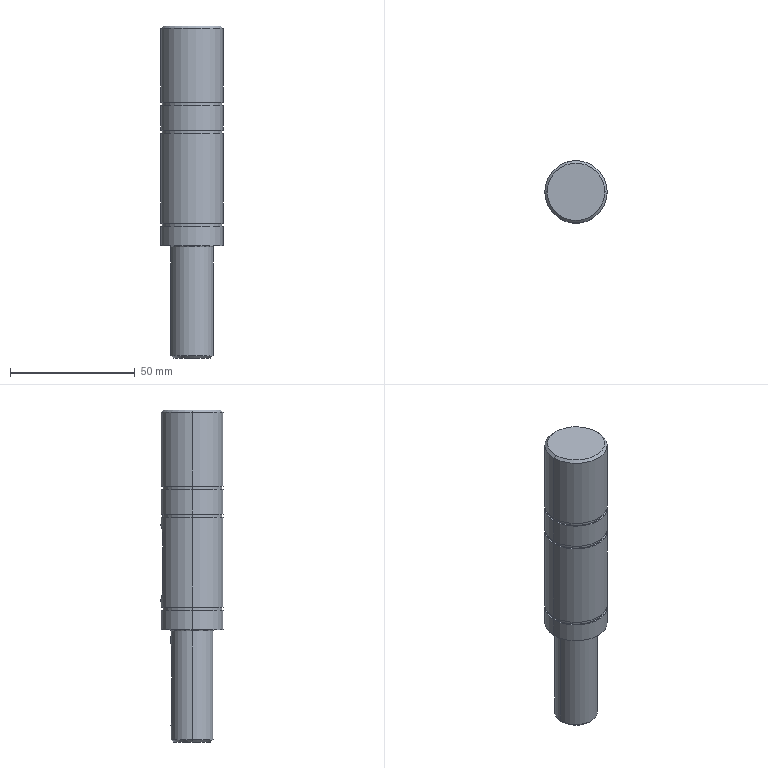Part | SolidWorks | features BaseBody 1 | 1 solid | 43 faces | box 25 x 25 x 133 mm | volume 51867 mm3 | cylinder 22 | plane 15 | cone 4 | spline 2 | commonest cylinder face diameters 25 x8 23.9 x6 5 x3 8 x3 17 x2
STEP:
#1=CARTESIAN_POINT('',(-8.5,0.,-0.5));
#2=VERTEX_POINT('',#1);
#3=CARTESIAN_POINT('',(8.5,0.,-0.5));
#4=VERTEX_POINT('',#3);
#5=CARTESIAN_POINT('',(0.,0.,-0.5));
#6=DIRECTION('',(0.,0.,-1.));
#7=DIRECTION('',(1.,0.,0.));
#8=AXIS2_PLACEMENT_3D('',#5,#6,#7);
#9=CIRCLE('',#8,8.5);
#10=EDGE_CURVE('',#2,#4,#9,.T.);
#11=ORIENTED_EDGE('',*,*,#10,.F.);
#12=CARTESIAN_POINT('',(-9.,0.,0.));
#13=VERTEX_POINT('',#12);
#14=CARTESIAN_POINT('',(-9.,0.,-0.5));
#15=DIRECTION('',(0.,-1.,0.));
#16=DIRECTION('',(-1.,0.,0.));
#17=AXIS2_PLACEMENT_3D('',#14,#15,#16);
#18=CIRCLE('',#17,0.5);
#19=EDGE_CURVE('',#2,#13,#18,.T.);
#20=ORIENTED_EDGE('',*,*,#19,.T.);
#21=CARTESIAN_POINT('',(9.,0.,0.));
#22=VERTEX_POINT('',#21);
#23=CARTESIAN_POINT('',(-9.,0.,0.));
#24=CARTESIAN_POINT('',(-9.,18.,0.));
#25=CARTESIAN_POINT('',(9.,18.,0.));
#26=CARTESIAN_POINT('',(9.,0.,0.));
#27=(BOUNDED_CURVE()B_SPLINE_CURVE(3,(#23,#24,#25,#26),.UNSPECIFIED.,.F.,.F.)B_SPLINE_CURVE_WITH_KNOTS((4,4),(0.,1.),.UNSPECIFIED.)CURVE()GEOMETRIC_REPRESENTATION_ITEM()RATIONAL_B_SPLINE_CURVE((1.,0.3333,0.3333,1.))REPRESENTATION_ITEM(''));
#28=EDGE_CURVE('',#13,#22,#27,.T.);
#29=ORIENTED_EDGE('',*,*,#28,.T.);
#30=CARTESIAN_POINT('',(9.,0.,-0.5));
#31=DIRECTION('',(0.,1.,0.));
#32=DIRECTION('',(1.,0.,0.));
#33=AXIS2_PLACEMENT_3D('',#30,#31,#32);
#34=CIRCLE('',#33,0.5);
#35=EDGE_CURVE('',#4,#22,#34,.T.);
#36=ORIENTED_EDGE('',*,*,#35,.F.);
#37=EDGE_LOOP('',(#11,#20,#29,#36));
#38=FACE_OUTER_BOUND('',#37,.T.);
#39=CARTESIAN_POINT('',(8.5,0.,-0.5));
#40=CARTESIAN_POINT('',(8.5,17.,-0.5));
#41=CARTESIAN_POINT('',(-8.5,17.,-0.5));
#42=CARTESIAN_POINT('',(-8.5,0.,-0.5));
#43=CARTESIAN_POINT('',(8.5,0.,-0.2071));
#44=CARTESIAN_POINT('',(8.5,17.,-0.2071));
#45=CARTESIAN_POINT('',(-8.5,17.,-0.2071));
#46=CARTESIAN_POINT('',(-8.5,0.,-0.2071));
#47=CARTESIAN_POINT('',(8.707,0.,0.));
#48=CARTESIAN_POINT('',(8.707,17.414,0.));
#49=CARTESIAN_POINT('',(-8.707,17.414,0.));
#50=CARTESIAN_POINT('',(-8.707,0.,0.));
#51=CARTESIAN_POINT('',(9.,0.,0.));
#52=CARTESIAN_POINT('',(9.,18.,0.));
#53=CARTESIAN_POINT('',(-9.,18.,0.));
#54=CARTESIAN_POINT('',(-9.,0.,0.));
#55=(BOUNDED_SURFACE()B_SPLINE_SURFACE(3,3,((#39,#40,#41,#42),(#43,#44,#45,#46),(#47,#48,#49,#50),(#51,#52,#53,#54)),.UNSPECIFIED.,.F.,.F.,.T.)B_SPLINE_SURFACE_WITH_KNOTS((4,4),(4,4),(0.,1.),(0.,1.),.UNSPECIFIED.)GEOMETRIC_REPRESENTATION_ITEM()RATIONAL_B_SPLINE_SURFACE(((1.,0.3333,0.3333,1.),(0.8047,0.2682,0.2682,0.8047),(0.8047,0.2682,0.2682,0.8047),(1.,0.3333,0.3333,1.)))REPRESENTATION_ITEM('')SURFACE());
#56=ADVANCED_FACE('',(#38),#55,.F.);
#57=CARTESIAN_POINT('',(-4.,11.843,16.));
#58=VERTEX_POINT('',#57);
#59=CARTESIAN_POINT('',(0.,12.5,12.));
#60=VERTEX_POINT('',#59);
#61=CARTESIAN_POINT('',(-4.,11.843,16.));
#62=CARTESIAN_POINT('',(-4.,11.843,15.734));
#63=CARTESIAN_POINT('',(-3.974,11.852,15.473));
#64=CARTESIAN_POINT('',(-3.871,11.886,14.96));
#65=CARTESIAN_POINT('',(-3.794,11.911,14.705));
#66=CARTESIAN_POINT('',(-3.592,11.973,14.221));
#67=CARTESIAN_POINT('',(-3.47,12.01,13.993));
#68=CARTESIAN_POINT('',(-3.18,12.09,13.559));
#69=CARTESIAN_POINT('',(-3.012,12.133,13.356));
#70=CARTESIAN_POINT('',(-2.646,12.218,12.989));
#71=CARTESIAN_POINT('',(-2.446,12.26,12.824));
#72=CARTESIAN_POINT('',(-2.01,12.339,12.532));
#73=CARTESIAN_POINT('',(-1.78,12.375,12.409));
#74=CARTESIAN_POINT('',(-1.3,12.435,12.208));
#75=CARTESIAN_POINT('',(-1.047,12.459,12.13));
#76=CARTESIAN_POINT('',(-0.5285,12.492,12.026));
#77=CARTESIAN_POINT('',(-0.266,12.5,12.));
#78=CARTESIAN_POINT('',(0.,12.5,12.));
#79=B_SPLINE_CURVE_WITH_KNOTS('',3,(#61,#62,#63,#64,#65,#66,#67,#68,#69,#70,#71,#72,#73,#74,#75,#76,#77,#78),.UNSPECIFIED.,.F.,.F.,(4,2,2,2,2,2,2,2,4),(-0.00629,-0.005504,-0.004718,-0.003932,-0.003145,-0.002359,-0.001573,-0.0007863,0.),.UNSPECIFIED.);
#80=EDGE_CURVE('',#58,#60,#79,.T.);
#81=ORIENTED_EDGE('',*,*,#80,.T.);
#82=CARTESIAN_POINT('',(4.,11.843,16.));
#83=VERTEX_POINT('',#82);
#84=CARTESIAN_POINT('',(0.,12.5,12.));
#85=CARTESIAN_POINT('',(0.266,12.5,12.));
#86=CARTESIAN_POINT('',(0.5272,12.492,12.026));
#87=CARTESIAN_POINT('',(1.041,12.459,12.129));
#88=CARTESIAN_POINT('',(1.296,12.435,12.207));
#89=CARTESIAN_POINT('',(1.779,12.375,12.408));
#90=CARTESIAN_POINT('',(2.008,12.34,12.531));
#91=CARTESIAN_POINT('',(2.441,12.261,12.821));
#92=CARTESIAN_POINT('',(2.645,12.218,12.988));
#93=CARTESIAN_POINT('',(3.011,12.133,13.354));
#94=CARTESIAN_POINT('',(3.176,12.091,13.554));
#95=CARTESIAN_POINT('',(3.469,12.01,13.991));
#96=CARTESIAN_POINT('',(3.592,11.973,14.22));
#97=CARTESIAN_POINT('',(3.792,11.911,14.7));
#98=CARTESIAN_POINT('',(3.87,11.886,14.954));
#99=CARTESIAN_POINT('',(3.974,11.852,15.472));
#100=CARTESIAN_POINT('',(4.,11.843,15.734));
#101=CARTESIAN_POINT('',(4.,11.843,16.));
#102=B_SPLINE_CURVE_WITH_KNOTS('',3,(#84,#85,#86,#87,#88,#89,#90,#91,#92,#93,#94,#95,#96,#97,#98,#99,#100,#101),.UNSPECIFIED.,.F.,.F.,(4,2,2,2,2,2,2,2,4),(0.,0.0007863,0.001573,0.002359,0.003145,0.003932,0.004718,0.005504,0.00629),.UNSPECIFIED.);
#103=EDGE_CURVE('',#60,#83,#102,.T.);
#104=ORIENTED_EDGE('',*,*,#103,.T.);
#105=CARTESIAN_POINT('',(4.,11.843,38.));
#106=VERTEX_POINT('',#105);
#107=CARTESIAN_POINT('',(4.,11.843,88.));
#108=DIRECTION('',(0.,0.,1.));
#109=VECTOR('',#108,1000.);
#110=LINE('',#107,#109);
#111=EDGE_CURVE('',#83,#106,#110,.T.);
#112=ORIENTED_EDGE('',*,*,#111,.T.);
#113=CARTESIAN_POINT('',(-4.,11.843,38.));
#114=VERTEX_POINT('',#113);
#115=CARTESIAN_POINT('',(4.,11.843,38.));
#116=CARTESIAN_POINT('',(4.,11.843,38.266));
#117=CARTESIAN_POINT('',(3.974,11.852,38.527));
#118=CARTESIAN_POINT('',(3.871,11.886,39.041));
#119=CARTESIAN_POINT('',(3.793,11.911,39.296));
#120=CARTESIAN_POINT('',(3.592,11.973,39.779));
#121=CARTESIAN_POINT('',(3.469,12.01,40.008));
#122=CARTESIAN_POINT('',(3.179,12.09,40.441));
#123=CARTESIAN_POINT('',(3.012,12.133,40.645));
#124=CARTESIAN_POINT('',(2.646,12.218,41.011));
#125=CARTESIAN_POINT('',(2.445,12.26,41.176));
#126=CARTESIAN_POINT('',(2.009,12.34,41.469));
#127=CARTESIAN_POINT('',(1.779,12.375,41.592));
#128=CARTESIAN_POINT('',(1.299,12.435,41.792));
#129=CARTESIAN_POINT('',(1.045,12.459,41.87));
#130=CARTESIAN_POINT('',(0.5276,12.492,41.974));
#131=CARTESIAN_POINT('',(0.2669,12.5,42.));
#132=CARTESIAN_POINT('',(-0.2587,12.5,42.));
#133=CARTESIAN_POINT('',(-0.5256,12.492,41.974));
#134=CARTESIAN_POINT('',(-1.04,12.459,41.871));
#135=CARTESIAN_POINT('',(-1.29,12.436,41.795));
#136=CARTESIAN_POINT('',(-1.777,12.375,41.593));
#137=CARTESIAN_POINT('',(-2.008,12.34,41.469));
#138=CARTESIAN_POINT('',(-2.44,12.262,41.18));
#139=CARTESIAN_POINT('',(-2.643,12.219,41.013));
#140=CARTESIAN_POINT('',(-3.012,12.133,40.645));
#141=CARTESIAN_POINT('',(-3.176,12.091,40.445));
#142=CARTESIAN_POINT('',(-3.466,12.011,40.013));
#143=CARTESIAN_POINT('',(-3.592,11.973,39.78));
#144=CARTESIAN_POINT('',(-3.792,11.911,39.298));
#145=CARTESIAN_POINT('',(-3.869,11.886,39.049));
#146=CARTESIAN_POINT('',(-3.973,11.852,38.532));
#147=CARTESIAN_POINT('',(-4.,11.843,38.266));
#148=CARTESIAN_POINT('',(-4.,11.843,38.));
#149=B_SPLINE_CURVE_WITH_KNOTS('',3,(#115,#116,#117,#118,#119,#120,#121,#122,#123,#124,#125,#126,#127,#128,#129,#130,#131,#132,#133,#134,#135,#136,#137,#138,#139,#140,#141,#142,#143,#144,#145,#146,#147,#148),.UNSPECIFIED.,.F.,.F.,(4,2,2,2,2,2,2,2,2,2,2,2,2,2,2,2,4),(0.,0.0007865,0.001573,0.00236,0.003146,0.003933,0.004719,0.005506,0.006292,0.007079,0.007865,0.008652,0.009438,0.01022,0.01101,0.0118,0.01258),.UNSPECIFIED.);
#150=EDGE_CURVE('',#106,#114,#149,.T.);
#151=ORIENTED_EDGE('',*,*,#150,.T.);
#152=CARTESIAN_POINT('',(-4.,11.843,88.));
#153=DIRECTION('',(0.,0.,-1.));
#154=VECTOR('',#153,1000.);
#155=LINE('',#152,#154);
#156=EDGE_CURVE('',#114,#58,#155,.T.);
#157=ORIENTED_EDGE('',*,*,#156,.T.);
#158=EDGE_LOOP('',(#81,#104,#112,#151,#157));
#159=FACE_BOUND('',#158,.T.);
#160=CARTESIAN_POINT('',(-12.5,0.,45.));
#161=VERTEX_POINT('',#160);
#162=CARTESIAN_POINT('',(12.5,0.,45.));
#163=VERTEX_POINT('',#162);
#164=CARTESIAN_POINT('',(0.,0.,45.));
#165=DIRECTION('',(0.,0.,-1.));
#166=DIRECTION('',(-1.,0.,0.));
#167=AXIS2_PLACEMENT_3D('',#164,#165,#166);
#168=CIRCLE('',#167,12.5);
#169=EDGE_CURVE('',#161,#163,#168,.T.);
#170=ORIENTED_EDGE('',*,*,#169,.T.);
#171=CARTESIAN_POINT('',(12.5,0.,9.));
#172=VERTEX_POINT('',#171);
#173=CARTESIAN_POINT('',(12.5,0.,88.));
#174=DIRECTION('',(0.,0.,-1.));
#175=VECTOR('',#174,1000.);
#176=LINE('',#173,#175);
#177=EDGE_CURVE('',#163,#172,#176,.T.);
#178=ORIENTED_EDGE('',*,*,#177,.T.);
#179=CARTESIAN_POINT('',(-12.5,0.,9.));
#180=VERTEX_POINT('',#179);
#181=CARTESIAN_POINT('',(0.,0.,9.));
#182=DIRECTION('',(0.,0.,1.));
#183=DIRECTION('',(-1.,0.,0.));
#184=AXIS2_PLACEMENT_3D('',#181,#182,#183);
#185=CIRCLE('',#184,12.5);
#186=EDGE_CURVE('',#172,#180,#185,.T.);
#187=ORIENTED_EDGE('',*,*,#186,.T.);
#188=CARTESIAN_POINT('',(-12.5,0.,88.));
#189=DIRECTION('',(0.,0.,-1.));
#190=VECTOR('',#189,1000.);
#191=LINE('',#188,#190);
#192=EDGE_CURVE('',#161,#180,#191,.T.);
#193=ORIENTED_EDGE('',*,*,#192,.F.);
#194=EDGE_LOOP('',(#170,#178,#187,#193));
#195=FACE_OUTER_BOUND('',#194,.T.);
#196=CARTESIAN_POINT('',(0.,0.,88.));
#197=DIRECTION('',(0.,0.,-1.));
#198=DIRECTION('',(-1.,0.,0.));
#199=AXIS2_PLACEMENT_3D('',#196,#197,#198);
#200=CYLINDRICAL_SURFACE('',#199,12.5);
#201=ADVANCED_FACE('',(#159,#195),#200,.T.);
#202=CARTESIAN_POINT('',(-11.95,0.,9.));
#203=VERTEX_POINT('',#202);
#204=CARTESIAN_POINT('',(11.95,0.,9.));
#205=VERTEX_POINT('',#204);
#206=CARTESIAN_POINT('',(0.,0.,9.));
#207=DIRECTION('',(0.,0.,-1.));
#208=DIRECTION('',(-1.,0.,0.));
#209=AXIS2_PLACEMENT_3D('',#206,#207,#208);
#210=CIRCLE('',#209,11.95);
#211=EDGE_CURVE('',#203,#205,#210,.T.);
#212=ORIENTED_EDGE('',*,*,#211,.T.);
#213=CARTESIAN_POINT('',(11.95,0.,7.7));
#214=VERTEX_POINT('',#213);
#215=CARTESIAN_POINT('',(11.95,0.,0.));
#216=DIRECTION('',(0.,0.,-1.));
#217=VECTOR('',#216,1000.);
#218=LINE('',#215,#217);
#219=EDGE_CURVE('',#205,#214,#218,.T.);
#220=ORIENTED_EDGE('',*,*,#219,.T.);
#221=CARTESIAN_POINT('',(-11.95,0.,7.7));
#222=VERTEX_POINT('',#221);
#223=CARTESIAN_POINT('',(0.,0.,7.7));
#224=DIRECTION('',(0.,0.,1.));
#225=DIRECTION('',(-1.,0.,0.));
#226=AXIS2_PLACEMENT_3D('',#223,#224,#225);
#227=CIRCLE('',#226,11.95);
#228=EDGE_CURVE('',#214,#222,#227,.T.);
#229=ORIENTED_EDGE('',*,*,#228,.T.);
#230=CARTESIAN_POINT('',(-11.95,0.,0.));
#231=DIRECTION('',(0.,0.,-1.));
#232=VECTOR('',#231,1000.);
#233=LINE('',#230,#232);
#234=EDGE_CURVE('',#203,#222,#233,.T.);
#235=ORIENTED_EDGE('',*,*,#234,.F.);
#236=EDGE_LOOP('',(#212,#220,#229,#235));
#237=FACE_OUTER_BOUND('',#236,.T.);
#238=CARTESIAN_POINT('',(0.,0.,0.));
#239=DIRECTION('',(0.,0.,-1.));
#240=DIRECTION('',(-1.,0.,0.));
#241=AXIS2_PLACEMENT_3D('',#238,#239,#240);
#242=CYLINDRICAL_SURFACE('',#241,11.95);
#243=ADVANCED_FACE('',(#237),#242,.T.);
#244=ORIENTED_EDGE('',*,*,#103,.F.);
#245=CARTESIAN_POINT('',(0.,8.5,12.));
#246=VERTEX_POINT('',#245);
#247=CARTESIAN_POINT('',(0.,12.5,12.));
#248=DIRECTION('',(0.,-1.,0.));
#249=VECTOR('',#248,1000.);
#250=LINE('',#247,#249);
#251=EDGE_CURVE('',#60,#246,#250,.T.);
#252=ORIENTED_EDGE('',*,*,#251,.T.);
#253=CARTESIAN_POINT('',(4.,8.5,16.));
#254=VERTEX_POINT('',#253);
#255=CARTESIAN_POINT('',(0.,8.5,16.));
#256=DIRECTION('',(0.,1.,0.));
#257=DIRECTION('',(0.,0.,-1.));
#258=AXIS2_PLACEMENT_3D('',#255,#256,#257);
#259=CIRCLE('',#258,4.);
#260=EDGE_CURVE('',#254,#246,#259,.T.);
#261=ORIENTED_EDGE('',*,*,#260,.F.);
#262=CARTESIAN_POINT('',(4.,12.5,16.));
#263=DIRECTION('',(0.,-1.,0.));
#264=VECTOR('',#263,1000.);
#265=LINE('',#262,#264);
#266=EDGE_CURVE('',#83,#254,#265,.T.);
#267=ORIENTED_EDGE('',*,*,#266,.F.);
#268=EDGE_LOOP('',(#244,#252,#261,#267));
#269=FACE_OUTER_BOUND('',#268,.T.);
#270=CARTESIAN_POINT('',(0.,12.5,16.));
#271=DIRECTION('',(0.,-1.,0.));
#272=DIRECTION('',(0.,0.,-1.));
#273=AXIS2_PLACEMENT_3D('',#270,#271,#272);
#274=CYLINDRICAL_SURFACE('',#273,4.);
#275=ADVANCED_FACE('',(#269),#274,.F.);
#276=CARTESIAN_POINT('',(-11.95,0.,46.3));
#277=VERTEX_POINT('',#276);
#278=CARTESIAN_POINT('',(11.95,0.,46.3));
#279=VERTEX_POINT('',#278);
#280=CARTESIAN_POINT('',(0.,0.,46.3));
#281=DIRECTION('',(0.,0.,-1.));
#282=DIRECTION('',(-1.,0.,0.));
#283=AXIS2_PLACEMENT_3D('',#280,#281,#282);
#284=CIRCLE('',#283,11.95);
#285=EDGE_CURVE('',#277,#279,#284,.T.);
#286=ORIENTED_EDGE('',*,*,#285,.T.);
#287=CARTESIAN_POINT('',(11.95,0.,45.));
#288=VERTEX_POINT('',#287);
#289=CARTESIAN_POINT('',(11.95,0.,0.));
#290=DIRECTION('',(0.,0.,-1.));
#291=VECTOR('',#290,1000.);
#292=LINE('',#289,#291);
#293=EDGE_CURVE('',#279,#288,#292,.T.);
#294=ORIENTED_EDGE('',*,*,#293,.T.);
#295=CARTESIAN_POINT('',(-11.95,0.,45.));
#296=VERTEX_POINT('',#295);
#297=CARTESIAN_POINT('',(0.,0.,45.));
#298=DIRECTION('',(0.,0.,1.));
#299=DIRECTION('',(-1.,0.,0.));
#300=AXIS2_PLACEMENT_3D('',#297,#298,#299);
#301=CIRCLE('',#300,11.95);
#302=EDGE_CURVE('',#288,#296,#301,.T.);
#303=ORIENTED_EDGE('',*,*,#302,.T.);
#304=CARTESIAN_POINT('',(-11.95,0.,0.));
#305=DIRECTION('',(0.,0.,-1.));
#306=VECTOR('',#305,1000.);
#307=LINE('',#304,#306);
#308=EDGE_CURVE('',#277,#296,#307,.T.);
#309=ORIENTED_EDGE('',*,*,#308,.F.);
#310=EDGE_LOOP('',(#286,#294,#303,#309));
#311=FACE_OUTER_BOUND('',#310,.T.);
#312=CARTESIAN_POINT('',(0.,0.,0.));
#313=DIRECTION('',(0.,0.,-1.));
#314=DIRECTION('',(-1.,0.,0.));
#315=AXIS2_PLACEMENT_3D('',#312,#313,#314);
#316=CYLINDRICAL_SURFACE('',#315,11.95);
#317=ADVANCED_FACE('',(#311),#316,.T.);
#318=CARTESIAN_POINT('',(-12.5,0.,7.7));
#319=VERTEX_POINT('',#318);
#320=CARTESIAN_POINT('',(12.5,0.,7.7));
#321=VERTEX_POINT('',#320);
#322=CARTESIAN_POINT('',(0.,0.,7.7));
#323=DIRECTION('',(0.,0.,-1.));
#324=DIRECTION('',(-1.,0.,0.));
#325=AXIS2_PLACEMENT_3D('',#322,#323,#324);
#326=CIRCLE('',#325,12.5);
#327=EDGE_CURVE('',#319,#321,#326,.T.);
#328=ORIENTED_EDGE('',*,*,#327,.T.);
#329=CARTESIAN_POINT('',(12.5,0.,0.));
#330=VERTEX_POINT('',#329);
#331=CARTESIAN_POINT('',(12.5,0.,88.));
#332=DIRECTION('',(0.,0.,-1.));
#333=VECTOR('',#332,1000.);
#334=LINE('',#331,#333);
#335=EDGE_CURVE('',#321,#330,#334,.T.);
#336=ORIENTED_EDGE('',*,*,#335,.T.);
#337=CARTESIAN_POINT('',(-12.5,0.,0.));
#338=VERTEX_POINT('',#337);
#339=CARTESIAN_POINT('',(0.,0.,0.));
#340=DIRECTION('',(0.,0.,1.));
#341=DIRECTION('',(-1.,0.,0.));
#342=AXIS2_PLACEMENT_3D('',#339,#340,#341);
#343=CIRCLE('',#342,12.5);
#344=EDGE_CURVE('',#330,#338,#343,.T.);
#345=ORIENTED_EDGE('',*,*,#344,.T.);
#346=CARTESIAN_POINT('',(-12.5,0.,88.));
#347=DIRECTION('',(0.,0.,-1.));
#348=VECTOR('',#347,1000.);
#349=LINE('',#346,#348);
#350=EDGE_CURVE('',#319,#338,#349,.T.);
#351=ORIENTED_EDGE('',*,*,#350,.F.);
#352=EDGE_LOOP('',(#328,#336,#345,#351));
#353=FACE_OUTER_BOUND('',#352,.T.);
#354=CARTESIAN_POINT('',(0.,0.,88.));
#355=DIRECTION('',(0.,0.,-1.));
#356=DIRECTION('',(-1.,0.,0.));
#357=AXIS2_PLACEMENT_3D('',#354,#355,#356);
#358=CYLINDRICAL_SURFACE('',#357,12.5);
#359=ADVANCED_FACE('',(#353),#358,.T.);
#360=CARTESIAN_POINT('',(-12.5,0.,56.2));
#361=VERTEX_POINT('',#360);
#362=CARTESIAN_POINT('',(12.5,0.,56.2));
#363=VERTEX_POINT('',#362);
#364=CARTESIAN_POINT('',(0.,0.,56.2));
#365=DIRECTION('',(0.,0.,-1.));
#366=DIRECTION('',(-1.,0.,0.));
#367=AXIS2_PLACEMENT_3D('',#364,#365,#366);
#368=CIRCLE('',#367,12.5);
#369=EDGE_CURVE('',#361,#363,#368,.T.);
#370=ORIENTED_EDGE('',*,*,#369,.T.);
#371=CARTESIAN_POINT('',(12.5,0.,46.3));
#372=VERTEX_POINT('',#371);
#373=CARTESIAN_POINT('',(12.5,0.,88.));
#374=DIRECTION('',(0.,0.,-1.));
#375=VECTOR('',#374,1000.);
#376=LINE('',#373,#375);
#377=EDGE_CURVE('',#363,#372,#376,.T.);
#378=ORIENTED_EDGE('',*,*,#377,.T.);
#379=CARTESIAN_POINT('',(-12.5,0.,46.3));
#380=VERTEX_POINT('',#379);
#381=CARTESIAN_POINT('',(0.,0.,46.3));
#382=DIRECTION('',(0.,0.,1.));
#383=DIRECTION('',(-1.,0.,0.));
#384=AXIS2_PLACEMENT_3D('',#381,#382,#383);
#385=CIRCLE('',#384,12.5);
#386=EDGE_CURVE('',#372,#380,#385,.T.);
#387=ORIENTED_EDGE('',*,*,#386,.T.);
#388=CARTESIAN_POINT('',(-12.5,0.,88.));
#389=DIRECTION('',(0.,0.,-1.));
#390=VECTOR('',#389,1000.);
#391=LINE('',#388,#390);
#392=EDGE_CURVE('',#361,#380,#391,.T.);
#393=ORIENTED_EDGE('',*,*,#392,.F.);
#394=EDGE_LOOP('',(#370,#378,#387,#393));
#395=FACE_OUTER_BOUND('',#394,.T.);
#396=CARTESIAN_POINT('',(0.,0.,88.));
#397=DIRECTION('',(0.,0.,-1.));
#398=DIRECTION('',(-1.,0.,0.));
#399=AXIS2_PLACEMENT_3D('',#396,#397,#398);
#400=CYLINDRICAL_SURFACE('',#399,12.5);
#401=ADVANCED_FACE('',(#395),#400,.T.);
#402=CARTESIAN_POINT('',(-11.95,0.,57.5));
#403=VERTEX_POINT('',#402);
#404=CARTESIAN_POINT('',(11.95,0.,57.5));
#405=VERTEX_POINT('',#404);
#406=CARTESIAN_POINT('',(0.,0.,57.5));
#407=DIRECTION('',(0.,0.,-1.));
#408=DIRECTION('',(-1.,0.,0.));
#409=AXIS2_PLACEMENT_3D('',#406,#407,#408);
#410=CIRCLE('',#409,11.95);
#411=EDGE_CURVE('',#403,#405,#410,.T.);
#412=ORIENTED_EDGE('',*,*,#411,.T.);
#413=CARTESIAN_POINT('',(11.95,0.,56.2));
#414=VERTEX_POINT('',#413);
#415=CARTESIAN_POINT('',(11.95,0.,0.));
#416=DIRECTION('',(0.,0.,-1.));
#417=VECTOR('',#416,1000.);
#418=LINE('',#415,#417);
#419=EDGE_CURVE('',#405,#414,#418,.T.);
#420=ORIENTED_EDGE('',*,*,#419,.T.);
#421=CARTESIAN_POINT('',(-11.95,0.,56.2));
#422=VERTEX_POINT('',#421);
#423=CARTESIAN_POINT('',(0.,0.,56.2));
#424=DIRECTION('',(0.,0.,1.));
#425=DIRECTION('',(-1.,0.,0.));
#426=AXIS2_PLACEMENT_3D('',#423,#424,#425);
#427=CIRCLE('',#426,11.95);
#428=EDGE_CURVE('',#414,#422,#427,.T.);
#429=ORIENTED_EDGE('',*,*,#428,.T.);
#430=CARTESIAN_POINT('',(-11.95,0.,0.));
#431=DIRECTION('',(0.,0.,-1.));
#432=VECTOR('',#431,1000.);
#433=LINE('',#430,#432);
#434=EDGE_CURVE('',#403,#422,#433,.T.);
#435=ORIENTED_EDGE('',*,*,#434,.F.);
#436=EDGE_LOOP('',(#412,#420,#429,#435));
#437=FACE_OUTER_BOUND('',#436,.T.);
#438=CARTESIAN_POINT('',(0.,0.,0.));
#439=DIRECTION('',(0.,0.,-1.));
#440=DIRECTION('',(-1.,0.,0.));
#441=AXIS2_PLACEMENT_3D('',#438,#439,#440);
#442=CYLINDRICAL_SURFACE('',#441,11.95);
#443=ADVANCED_FACE('',(#437),#442,.T.);
#444=CARTESIAN_POINT('',(-2.5,8.124,-8.));
#445=VERTEX_POINT('',#444);
#446=CARTESIAN_POINT('',(-2.5,8.124,-36.));
#447=VERTEX_POINT('',#446);
#448=CARTESIAN_POINT('',(-2.5,8.124,-45.));
#449=DIRECTION('',(0.,0.,-1.));
#450=VECTOR('',#449,1000.);
#451=LINE('',#448,#450);
#452=EDGE_CURVE('',#445,#447,#451,.T.);
#453=ORIENTED_EDGE('',*,*,#452,.T.);
#454=CARTESIAN_POINT('',(0.,8.5,-38.5));
#455=VERTEX_POINT('',#454);
#456=CARTESIAN_POINT('',(-2.5,8.124,-36.));
#457=CARTESIAN_POINT('',(-2.5,8.124,-36.166));
#458=CARTESIAN_POINT('',(-2.484,8.129,-36.329));
#459=CARTESIAN_POINT('',(-2.42,8.148,-36.65));
#460=CARTESIAN_POINT('',(-2.371,8.163,-36.809));
#461=CARTESIAN_POINT('',(-2.246,8.198,-37.111));
#462=CARTESIAN_POINT('',(-2.169,8.219,-37.254));
#463=CARTESIAN_POINT('',(-1.988,8.265,-37.525));
#464=CARTESIAN_POINT('',(-1.883,8.29,-37.653));
#465=CARTESIAN_POINT('',(-1.539,8.363,-37.996));
#466=CARTESIAN_POINT('',(-1.262,8.411,-38.182));
#467=CARTESIAN_POINT('',(-0.8118,8.462,-38.37));
#468=CARTESIAN_POINT('',(-0.6536,8.476,-38.419));
#469=CARTESIAN_POINT('',(-0.33,8.495,-38.484));
#470=CARTESIAN_POINT('',(-0.1661,8.5,-38.5));
#471=CARTESIAN_POINT('',(0.,8.5,-38.5));
#472=B_SPLINE_CURVE_WITH_KNOTS('',3,(#456,#457,#458,#459,#460,#461,#462,#463,#464,#465,#466,#467,#468,#469,#470,#471),.UNSPECIFIED.,.F.,.F.,(4,2,2,2,2,2,2,4),(0.,0.0004909,0.0009818,0.001473,0.001964,0.002945,0.003436,0.003927),.UNSPECIFIED.);
#473=EDGE_CURVE('',#447,#455,#472,.T.);
#474=ORIENTED_EDGE('',*,*,#473,.T.);
#475=CARTESIAN_POINT('',(2.5,8.124,-36.));
#476=VERTEX_POINT('',#475);
#477=CARTESIAN_POINT('',(0.,8.5,-38.5));
#478=CARTESIAN_POINT('',(0.1661,8.5,-38.5));
#479=CARTESIAN_POINT('',(0.3292,8.495,-38.484));
#480=CARTESIAN_POINT('',(0.6498,8.477,-38.42));
#481=CARTESIAN_POINT('',(0.809,8.463,-38.371));
#482=CARTESIAN_POINT('',(1.111,8.428,-38.245));
#483=CARTESIAN_POINT('',(1.254,8.408,-38.169));
#484=CARTESIAN_POINT('',(1.525,8.363,-37.987));
#485=CARTESIAN_POINT('',(1.653,8.339,-37.883));
#486=CARTESIAN_POINT('',(1.997,8.265,-37.539));
#487=CARTESIAN_POINT('',(2.183,8.216,-37.262));
#488=CARTESIAN_POINT('',(2.37,8.163,-36.812));
#489=CARTESIAN_POINT('',(2.419,8.149,-36.654));
#490=CARTESIAN_POINT('',(2.484,8.129,-36.33));
#491=CARTESIAN_POINT('',(2.5,8.124,-36.166));
#492=CARTESIAN_POINT('',(2.5,8.124,-36.));
#493=B_SPLINE_CURVE_WITH_KNOTS('',3,(#477,#478,#479,#480,#481,#482,#483,#484,#485,#486,#487,#488,#489,#490,#491,#492),.UNSPECIFIED.,.F.,.F.,(4,2,2,2,2,2,2,4),(0.003927,0.004418,0.004909,0.0054,0.005891,0.006873,0.007364,0.007855),.UNSPECIFIED.);
#494=EDGE_CURVE('',#455,#476,#493,.T.);
#495=ORIENTED_EDGE('',*,*,#494,.T.);
#496=CARTESIAN_POINT('',(2.5,8.124,-8.));
#497=VERTEX_POINT('',#496);
#498=CARTESIAN_POINT('',(2.5,8.124,-45.));
#499=DIRECTION('',(0.,0.,1.));
#500=VECTOR('',#499,1000.);
#501=LINE('',#498,#500);
#502=EDGE_CURVE('',#476,#497,#501,.T.);
#503=ORIENTED_EDGE('',*,*,#502,.T.);
#504=CARTESIAN_POINT('',(2.5,8.124,-8.));
#505=CARTESIAN_POINT('',(2.5,8.124,-7.834));
#506=CARTESIAN_POINT('',(2.484,8.129,-7.671));
#507=CARTESIAN_POINT('',(2.42,8.148,-7.35));
#508=CARTESIAN_POINT('',(2.371,8.163,-7.191));
#509=CARTESIAN_POINT('',(2.245,8.198,-6.889));
#510=CARTESIAN_POINT('',(2.169,8.219,-6.745));
#511=CARTESIAN_POINT('',(1.987,8.265,-6.474));
#512=CARTESIAN_POINT('',(1.882,8.29,-6.347));
#513=CARTESIAN_POINT('',(1.539,8.363,-6.003));
#514=CARTESIAN_POINT('',(1.261,8.411,-5.817));
#515=CARTESIAN_POINT('',(0.8108,8.463,-5.63));
#516=CARTESIAN_POINT('',(0.6524,8.476,-5.581));
#517=CARTESIAN_POINT('',(0.3293,8.495,-5.516));
#518=CARTESIAN_POINT('',(0.1665,8.5,-5.5));
#519=CARTESIAN_POINT('',(-0.1616,8.5,-5.5));
#520=CARTESIAN_POINT('',(-0.3283,8.495,-5.516));
#521=CARTESIAN_POINT('',(-0.6497,8.477,-5.58));
#522=CARTESIAN_POINT('',(-0.806,8.463,-5.628));
#523=CARTESIAN_POINT('',(-1.262,8.411,-5.817));
#524=CARTESIAN_POINT('',(-1.536,8.363,-6.001));
#525=CARTESIAN_POINT('',(-1.883,8.29,-6.347));
#526=CARTESIAN_POINT('',(-1.985,8.265,-6.472));
#527=CARTESIAN_POINT('',(-2.167,8.22,-6.742));
#528=CARTESIAN_POINT('',(-2.245,8.198,-6.888));
#529=CARTESIAN_POINT('',(-2.371,8.163,-7.189));
#530=CARTESIAN_POINT('',(-2.418,8.149,-7.345));
#531=CARTESIAN_POINT('',(-2.483,8.129,-7.668));
#532=CARTESIAN_POINT('',(-2.5,8.124,-7.834));
#533=CARTESIAN_POINT('',(-2.5,8.124,-8.));
#534=B_SPLINE_CURVE_WITH_KNOTS('',3,(#504,#505,#506,#507,#508,#509,#510,#511,#512,#513,#514,#515,#516,#517,#518,#519,#520,#521,#522,#523,#524,#525,#526,#527,#528,#529,#530,#531,#532,#533),.UNSPECIFIED.,.F.,.F.,(4,2,2,2,2,2,2,2,2,2,2,2,2,2,4),(0.,0.0004911,0.0009821,0.001473,0.001964,0.002946,0.003437,0.003929,0.00442,0.004911,0.005893,0.006384,0.006875,0.007366,0.007857),.UNSPECIFIED.);
#535=EDGE_CURVE('',#497,#445,#534,.T.);
#536=ORIENTED_EDGE('',*,*,#535,.T.);
#537=EDGE_LOOP('',(#453,#474,#495,#503,#536));
#538=FACE_BOUND('',#537,.T.);
#539=CARTESIAN_POINT('',(8.5,0.,-44.));
#540=VERTEX_POINT('',#539);
#541=CARTESIAN_POINT('',(-8.5,0.,-44.));
#542=VERTEX_POINT('',#541);
#543=CARTESIAN_POINT('',(0.,0.,-44.));
#544=DIRECTION('',(0.,0.,1.));
#545=DIRECTION('',(1.,0.,0.));
#546=AXIS2_PLACEMENT_3D('',#543,#544,#545);
#547=CIRCLE('',#546,8.5);
#548=EDGE_CURVE('',#540,#542,#547,.T.);
#549=ORIENTED_EDGE('',*,*,#548,.T.);
#550=CARTESIAN_POINT('',(-8.5,0.,-45.));
#551=DIRECTION('',(0.,0.,1.));
#552=VECTOR('',#551,1000.);
#553=LINE('',#550,#552);
#554=EDGE_CURVE('',#542,#2,#553,.T.);
#555=ORIENTED_EDGE('',*,*,#554,.T.);
#556=ORIENTED_EDGE('',*,*,#10,.T.);
#557=CARTESIAN_POINT('',(8.5,0.,-45.));
#558=DIRECTION('',(0.,0.,1.));
#559=VECTOR('',#558,1000.);
#560=LINE('',#557,#559);
#561=EDGE_CURVE('',#540,#4,#560,.T.);
#562=ORIENTED_EDGE('',*,*,#561,.F.);
#563=EDGE_LOOP('',(#549,#555,#556,#562));
#564=FACE_OUTER_BOUND('',#563,.T.);
#565=CARTESIAN_POINT('',(0.,0.,-45.));
#566=DIRECTION('',(0.,0.,1.));
#567=DIRECTION('',(1.,0.,0.));
#568=AXIS2_PLACEMENT_3D('',#565,#566,#567);
#569=CYLINDRICAL_SURFACE('',#568,8.5);
#570=ADVANCED_FACE('',(#538,#564),#569,.T.);
#571=CARTESIAN_POINT('',(7.5,0.,-45.));
#572=VERTEX_POINT('',#571);
#573=CARTESIAN_POINT('',(-7.5,0.,-45.));
#574=VERTEX_POINT('',#573);
#575=CARTESIAN_POINT('',(0.,0.,-45.));
#576=DIRECTION('',(0.,0.,1.));
#577=DIRECTION('',(1.,0.,0.));
#578=AXIS2_PLACEMENT_3D('',#575,#576,#577);
#579=CIRCLE('',#578,7.5);
#580=EDGE_CURVE('',#572,#574,#579,.T.);
#581=ORIENTED_EDGE('',*,*,#580,.T.);
#582=CARTESIAN_POINT('',(-8.5,0.,-44.));
#583=DIRECTION('',(-0.7071,0.,0.7071));
#584=VECTOR('',#583,1000.);
#585=LINE('',#582,#584);
#586=EDGE_CURVE('',#574,#542,#585,.T.);
#587=ORIENTED_EDGE('',*,*,#586,.T.);
#588=ORIENTED_EDGE('',*,*,#548,.F.);
#589=CARTESIAN_POINT('',(8.5,0.,-44.));
#590=DIRECTION('',(0.7071,0.,0.7071));
#591=VECTOR('',#590,1000.);
#592=LINE('',#589,#591);
#593=EDGE_CURVE('',#572,#540,#592,.T.);
#594=ORIENTED_EDGE('',*,*,#593,.F.);
#595=EDGE_LOOP('',(#581,#587,#588,#594));
#596=FACE_OUTER_BOUND('',#595,.T.);
#597=CARTESIAN_POINT('',(0.,0.,-44.));
#598=DIRECTION('',(0.,0.,1.));
#599=DIRECTION('',(1.,0.,0.));
#600=AXIS2_PLACEMENT_3D('',#597,#598,#599);
#601=CONICAL_SURFACE('',#600,8.5,0.7854);
#602=ADVANCED_FACE('',(#596),#601,.T.);
#603=ORIENTED_EDGE('',*,*,#494,.F.);
#604=CARTESIAN_POINT('',(0.,5.5,-38.5));
#605=VERTEX_POINT('',#604);
#606=CARTESIAN_POINT('',(0.,12.5,-38.5));
#607=DIRECTION('',(0.,-1.,0.));
#608=VECTOR('',#607,1000.);
#609=LINE('',#606,#608);
#610=EDGE_CURVE('',#455,#605,#609,.T.);
#611=ORIENTED_EDGE('',*,*,#610,.T.);
#612=CARTESIAN_POINT('',(2.5,5.5,-36.));
#613=VERTEX_POINT('',#612);
#614=CARTESIAN_POINT('',(0.,5.5,-36.));
#615=DIRECTION('',(0.,1.,0.));
#616=DIRECTION('',(0.,0.,-1.));
#617=AXIS2_PLACEMENT_3D('',#614,#615,#616);
#618=CIRCLE('',#617,2.5);
#619=EDGE_CURVE('',#613,#605,#618,.T.);
#620=ORIENTED_EDGE('',*,*,#619,.F.);
#621=CARTESIAN_POINT('',(2.5,12.5,-36.));
#622=DIRECTION('',(0.,-1.,0.));
#623=VECTOR('',#622,1000.);
#624=LINE('',#621,#623);
#625=EDGE_CURVE('',#476,#613,#624,.T.);
#626=ORIENTED_EDGE('',*,*,#625,.F.);
#627=EDGE_LOOP('',(#603,#611,#620,#626));
#628=FACE_OUTER_BOUND('',#627,.T.);
#629=CARTESIAN_POINT('',(0.,12.5,-36.));
#630=DIRECTION('',(0.,-1.,0.));
#631=DIRECTION('',(0.,0.,-1.));
#632=AXIS2_PLACEMENT_3D('',#629,#630,#631);
#633=CYLINDRICAL_SURFACE('',#632,2.5);
#634=ADVANCED_FACE('',(#628),#633,.F.);
#635=CARTESIAN_POINT('',(-12.5,0.,87.));
#636=VERTEX_POINT('',#635);
#637=CARTESIAN_POINT('',(12.5,0.,87.));
#638=VERTEX_POINT('',#637);
#639=CARTESIAN_POINT('',(0.,0.,87.));
#640=DIRECTION('',(0.,0.,-1.));
#641=DIRECTION('',(-1.,0.,0.));
#642=AXIS2_PLACEMENT_3D('',#639,#640,#641);
#643=CIRCLE('',#642,12.5);
#644=EDGE_CURVE('',#636,#638,#643,.T.);
#645=ORIENTED_EDGE('',*,*,#644,.T.);
#646=CARTESIAN_POINT('',(12.5,0.,57.5));
#647=VERTEX_POINT('',#646);
#648=CARTESIAN_POINT('',(12.5,0.,88.));
#649=DIRECTION('',(0.,0.,-1.));
#650=VECTOR('',#649,1000.);
#651=LINE('',#648,#650);
#652=EDGE_CURVE('',#638,#647,#651,.T.);
#653=ORIENTED_EDGE('',*,*,#652,.T.);
#654=CARTESIAN_POINT('',(-12.5,0.,57.5));
#655=VERTEX_POINT('',#654);
#656=CARTESIAN_POINT('',(0.,0.,57.5));
#657=DIRECTION('',(0.,0.,1.));
#658=DIRECTION('',(-1.,0.,0.));
#659=AXIS2_PLACEMENT_3D('',#656,#657,#658);
#660=CIRCLE('',#659,12.5);
#661=EDGE_CURVE('',#647,#655,#660,.T.);
#662=ORIENTED_EDGE('',*,*,#661,.T.);
#663=CARTESIAN_POINT('',(-12.5,0.,88.));
#664=DIRECTION('',(0.,0.,-1.));
#665=VECTOR('',#664,1000.);
#666=LINE('',#663,#665);
#667=EDGE_CURVE('',#636,#655,#666,.T.);
#668=ORIENTED_EDGE('',*,*,#667,.F.);
#669=EDGE_LOOP('',(#645,#653,#662,#668));
#670=FACE_OUTER_BOUND('',#669,.T.);
#671=CARTESIAN_POINT('',(0.,0.,88.));
#672=DIRECTION('',(0.,0.,-1.));
#673=DIRECTION('',(-1.,0.,0.));
#674=AXIS2_PLACEMENT_3D('',#671,#672,#673);
#675=CYLINDRICAL_SURFACE('',#674,12.5);
#676=ADVANCED_FACE('',(#670),#675,.T.);
#677=CARTESIAN_POINT('',(-11.5,0.,88.));
#678=VERTEX_POINT('',#677);
#679=CARTESIAN_POINT('',(11.5,0.,88.));
#680=VERTEX_POINT('',#679);
#681=CARTESIAN_POINT('',(0.,0.,88.));
#682=DIRECTION('',(0.,0.,-1.));
#683=DIRECTION('',(-1.,0.,0.));
#684=AXIS2_PLACEMENT_3D('',#681,#682,#683);
#685=CIRCLE('',#684,11.5);
#686=EDGE_CURVE('',#678,#680,#685,.T.);
#687=ORIENTED_EDGE('',*,*,#686,.T.);
#688=CARTESIAN_POINT('',(12.5,0.,87.));
#689=DIRECTION('',(0.7071,0.,-0.7071));
#690=VECTOR('',#689,1000.);
#691=LINE('',#688,#690);
#692=EDGE_CURVE('',#680,#638,#691,.T.);
#693=ORIENTED_EDGE('',*,*,#692,.T.);
#694=ORIENTED_EDGE('',*,*,#644,.F.);
#695=CARTESIAN_POINT('',(-12.5,0.,87.));
#696=DIRECTION('',(-0.7071,0.,-0.7071));
#697=VECTOR('',#696,1000.);
#698=LINE('',#695,#697);
#699=EDGE_CURVE('',#678,#636,#698,.T.);
#700=ORIENTED_EDGE('',*,*,#699,.F.);
#701=EDGE_LOOP('',(#687,#693,#694,#700));
#702=FACE_OUTER_BOUND('',#701,.T.);
#703=CARTESIAN_POINT('',(0.,0.,87.));
#704=DIRECTION('',(0.,0.,-1.));
#705=DIRECTION('',(-1.,0.,0.));
#706=AXIS2_PLACEMENT_3D('',#703,#704,#705);
#707=CONICAL_SURFACE('',#706,12.5,0.7854);
#708=ADVANCED_FACE('',(#702),#707,.T.);
#709=ORIENTED_EDGE('',*,*,#177,.F.);
#710=CARTESIAN_POINT('',(0.,0.,45.));
#711=DIRECTION('',(0.,0.,-1.));
#712=DIRECTION('',(-1.,0.,0.));
#713=AXIS2_PLACEMENT_3D('',#710,#711,#712);
#714=CIRCLE('',#713,12.5);
#715=EDGE_CURVE('',#163,#161,#714,.T.);
#716=ORIENTED_EDGE('',*,*,#715,.T.);
#717=ORIENTED_EDGE('',*,*,#192,.T.);
#718=CARTESIAN_POINT('',(0.,0.,9.));
#719=DIRECTION('',(0.,0.,1.));
#720=DIRECTION('',(-1.,0.,0.));
#721=AXIS2_PLACEMENT_3D('',#718,#719,#720);
#722=CIRCLE('',#721,12.5);
#723=EDGE_CURVE('',#180,#172,#722,.T.);
#724=ORIENTED_EDGE('',*,*,#723,.T.);
#725=EDGE_LOOP('',(#709,#716,#717,#724));
#726=FACE_OUTER_BOUND('',#725,.T.);
#727=CARTESIAN_POINT('',(0.,0.,88.));
#728=DIRECTION('',(0.,0.,-1.));
#729=DIRECTION('',(-1.,0.,0.));
#730=AXIS2_PLACEMENT_3D('',#727,#728,#729);
#731=CYLINDRICAL_SURFACE('',#730,12.5);
#732=ADVANCED_FACE('',(#726),#731,.T.);
#733=ORIENTED_EDGE('',*,*,#723,.F.);
#734=ORIENTED_EDGE('',*,*,#186,.F.);
#735=EDGE_LOOP('',(#733,#734));
#736=FACE_OUTER_BOUND('',#735,.T.);
#737=ORIENTED_EDGE('',*,*,#211,.F.);
#738=CARTESIAN_POINT('',(0.,0.,9.));
#739=DIRECTION('',(0.,0.,-1.));
#740=DIRECTION('',(-1.,0.,0.));
#741=AXIS2_PLACEMENT_3D('',#738,#739,#740);
#742=CIRCLE('',#741,11.95);
#743=EDGE_CURVE('',#205,#203,#742,.T.);
#744=ORIENTED_EDGE('',*,*,#743,.F.);
#745=EDGE_LOOP('',(#737,#744));
#746=FACE_BOUND('',#745,.T.);
#747=CARTESIAN_POINT('',(-11.95,0.,9.));
#748=DIRECTION('',(0.,0.,1.));
#749=DIRECTION('',(1.,0.,0.));
#750=AXIS2_PLACEMENT_3D('',#747,#748,#749);
#751=PLANE('',#750);
#752=ADVANCED_FACE('',(#736,#746),#751,.F.);
#753=ORIENTED_EDGE('',*,*,#169,.F.);
#754=ORIENTED_EDGE('',*,*,#715,.F.);
#755=EDGE_LOOP('',(#753,#754));
#756=FACE_OUTER_BOUND('',#755,.T.);
#757=CARTESIAN_POINT('',(0.,0.,45.));
#758=DIRECTION('',(0.,0.,1.));
#759=DIRECTION('',(-1.,0.,0.));
#760=AXIS2_PLACEMENT_3D('',#757,#758,#759);
#761=CIRCLE('',#760,11.95);
#762=EDGE_CURVE('',#296,#288,#761,.T.);
#763=ORIENTED_EDGE('',*,*,#762,.F.);
#764=ORIENTED_EDGE('',*,*,#302,.F.);
#765=EDGE_LOOP('',(#763,#764));
#766=FACE_BOUND('',#765,.T.);
#767=CARTESIAN_POINT('',(-17.505,0.,45.));
#768=DIRECTION('',(0.,0.,-1.));
#769=DIRECTION('',(-1.,0.,0.));
#770=AXIS2_PLACEMENT_3D('',#767,#768,#769);
#771=PLANE('',#770);
#772=ADVANCED_FACE('',(#756,#766),#771,.F.);
#773=ORIENTED_EDGE('',*,*,#219,.F.);
#774=ORIENTED_EDGE('',*,*,#743,.T.);
#775=ORIENTED_EDGE('',*,*,#234,.T.);
#776=CARTESIAN_POINT('',(0.,0.,7.7));
#777=DIRECTION('',(0.,0.,1.));
#778=DIRECTION('',(-1.,0.,0.));
#779=AXIS2_PLACEMENT_3D('',#776,#777,#778);
#780=CIRCLE('',#779,11.95);
#781=EDGE_CURVE('',#222,#214,#780,.T.);
#782=ORIENTED_EDGE('',*,*,#781,.T.);
#783=EDGE_LOOP('',(#773,#774,#775,#782));
#784=FACE_OUTER_BOUND('',#783,.T.);
#785=CARTESIAN_POINT('',(0.,0.,0.));
#786=DIRECTION('',(0.,0.,-1.));
#787=DIRECTION('',(-1.,0.,0.));
#788=AXIS2_PLACEMENT_3D('',#785,#786,#787);
#789=CYLINDRICAL_SURFACE('',#788,11.95);
#790=ADVANCED_FACE('',(#784),#789,.T.);
#791=CARTESIAN_POINT('',(4.,8.5,38.));
#792=VERTEX_POINT('',#791);
#793=CARTESIAN_POINT('',(4.,8.5,16.));
#794=DIRECTION('',(0.,0.,1.));
#795=VECTOR('',#794,1000.);
#796=LINE('',#793,#795);
#797=EDGE_CURVE('',#254,#792,#796,.T.);
#798=ORIENTED_EDGE('',*,*,#797,.T.);
#799=CARTESIAN_POINT('',(4.,12.5,38.));
#800=DIRECTION('',(0.,1.,0.));
#801=VECTOR('',#800,1000.);
#802=LINE('',#799,#801);
#803=EDGE_CURVE('',#792,#106,#802,.T.);
#804=ORIENTED_EDGE('',*,*,#803,.T.);
#805=ORIENTED_EDGE('',*,*,#111,.F.);
#806=ORIENTED_EDGE('',*,*,#266,.T.);
#807=EDGE_LOOP('',(#798,#804,#805,#806));
#808=FACE_OUTER_BOUND('',#807,.T.);
#809=CARTESIAN_POINT('',(4.,12.5,16.));
#810=DIRECTION('',(-1.,0.,0.));
#811=DIRECTION('',(0.,0.,1.));
#812=AXIS2_PLACEMENT_3D('',#809,#810,#811);
#813=PLANE('',#812);
#814=ADVANCED_FACE('',(#808),#813,.T.);
#815=ORIENTED_EDGE('',*,*,#251,.F.);
#816=ORIENTED_EDGE('',*,*,#80,.F.);
#817=CARTESIAN_POINT('',(-4.,8.5,16.));
#818=VERTEX_POINT('',#817);
#819=CARTESIAN_POINT('',(-4.,12.5,16.));
#820=DIRECTION('',(0.,1.,0.));
#821=VECTOR('',#820,1000.);
#822=LINE('',#819,#821);
#823=EDGE_CURVE('',#818,#58,#822,.T.);
#824=ORIENTED_EDGE('',*,*,#823,.F.);
#825=CARTESIAN_POINT('',(0.,8.5,16.));
#826=DIRECTION('',(0.,1.,0.));
#827=DIRECTION('',(0.,0.,-1.));
#828=AXIS2_PLACEMENT_3D('',#825,#826,#827);
#829=CIRCLE('',#828,4.);
#830=EDGE_CURVE('',#246,#818,#829,.T.);
#831=ORIENTED_EDGE('',*,*,#830,.F.);
#832=EDGE_LOOP('',(#815,#816,#824,#831));
#833=FACE_OUTER_BOUND('',#832,.T.);
#834=CARTESIAN_POINT('',(0.,12.5,16.));
#835=DIRECTION('',(0.,-1.,0.));
#836=DIRECTION('',(0.,0.,-1.));
#837=AXIS2_PLACEMENT_3D('',#834,#835,#836);
#838=CYLINDRICAL_SURFACE('',#837,4.);
#839=ADVANCED_FACE('',(#833),#838,.F.);
#840=CARTESIAN_POINT('',(-4.,8.5,38.));
#841=VERTEX_POINT('',#840);
#842=CARTESIAN_POINT('',(-4.,8.5,16.));
#843=DIRECTION('',(0.,0.,-1.));
#844=VECTOR('',#843,1000.);
#845=LINE('',#842,#844);
#846=EDGE_CURVE('',#841,#818,#845,.T.);
#847=ORIENTED_EDGE('',*,*,#846,.T.);
#848=ORIENTED_EDGE('',*,*,#823,.T.);
#849=ORIENTED_EDGE('',*,*,#156,.F.);
#850=CARTESIAN_POINT('',(-4.,12.5,38.));
#851=DIRECTION('',(0.,-1.,0.));
#852=VECTOR('',#851,1000.);
#853=LINE('',#850,#852);
#854=EDGE_CURVE('',#114,#841,#853,.T.);
#855=ORIENTED_EDGE('',*,*,#854,.T.);
#856=EDGE_LOOP('',(#847,#848,#849,#855));
#857=FACE_OUTER_BOUND('',#856,.T.);
#858=CARTESIAN_POINT('',(-4.,12.5,16.));
#859=DIRECTION('',(1.,0.,0.));
#860=DIRECTION('',(0.,0.,-1.));
#861=AXIS2_PLACEMENT_3D('',#858,#859,#860);
#862=PLANE('',#861);
#863=ADVANCED_FACE('',(#857),#862,.T.);
#864=ORIENTED_EDGE('',*,*,#150,.F.);
#865=ORIENTED_EDGE('',*,*,#803,.F.);
#866=CARTESIAN_POINT('',(0.,8.5,38.));
#867=DIRECTION('',(0.,1.,0.));
#868=DIRECTION('',(0.,0.,-1.));
#869=AXIS2_PLACEMENT_3D('',#866,#867,#868);
#870=CIRCLE('',#869,4.);
#871=EDGE_CURVE('',#841,#792,#870,.T.);
#872=ORIENTED_EDGE('',*,*,#871,.F.);
#873=ORIENTED_EDGE('',*,*,#854,.F.);
#874=EDGE_LOOP('',(#864,#865,#872,#873));
#875=FACE_OUTER_BOUND('',#874,.T.);
#876=CARTESIAN_POINT('',(0.,12.5,38.));
#877=DIRECTION('',(0.,-1.,0.));
#878=DIRECTION('',(0.,0.,-1.));
#879=AXIS2_PLACEMENT_3D('',#876,#877,#878);
#880=CYLINDRICAL_SURFACE('',#879,4.);
#881=ADVANCED_FACE('',(#875),#880,.F.);
#882=ORIENTED_EDGE('',*,*,#293,.F.);
#883=CARTESIAN_POINT('',(0.,0.,46.3));
#884=DIRECTION('',(0.,0.,-1.));
#885=DIRECTION('',(-1.,0.,0.));
#886=AXIS2_PLACEMENT_3D('',#883,#884,#885);
#887=CIRCLE('',#886,11.95);
#888=EDGE_CURVE('',#279,#277,#887,.T.);
#889=ORIENTED_EDGE('',*,*,#888,.T.);
#890=ORIENTED_EDGE('',*,*,#308,.T.);
#891=ORIENTED_EDGE('',*,*,#762,.T.);
#892=EDGE_LOOP('',(#882,#889,#890,#891));
#893=FACE_OUTER_BOUND('',#892,.T.);
#894=CARTESIAN_POINT('',(0.,0.,0.));
#895=DIRECTION('',(0.,0.,-1.));
#896=DIRECTION('',(-1.,0.,0.));
#897=AXIS2_PLACEMENT_3D('',#894,#895,#896);
#898=CYLINDRICAL_SURFACE('',#897,11.95);
#899=ADVANCED_FACE('',(#893),#898,.T.);
#900=ORIENTED_EDGE('',*,*,#327,.F.);
#901=CARTESIAN_POINT('',(0.,0.,7.7));
#902=DIRECTION('',(0.,0.,-1.));
#903=DIRECTION('',(-1.,0.,0.));
#904=AXIS2_PLACEMENT_3D('',#901,#902,#903);
#905=CIRCLE('',#904,12.5);
#906=EDGE_CURVE('',#321,#319,#905,.T.);
#907=ORIENTED_EDGE('',*,*,#906,.F.);
#908=EDGE_LOOP('',(#900,#907));
#909=FACE_OUTER_BOUND('',#908,.T.);
#910=ORIENTED_EDGE('',*,*,#781,.F.);
#911=ORIENTED_EDGE('',*,*,#228,.F.);
#912=EDGE_LOOP('',(#910,#911));
#913=FACE_BOUND('',#912,.T.);
#914=CARTESIAN_POINT('',(-11.95,0.,7.7));
#915=DIRECTION('',(0.,0.,-1.));
#916=DIRECTION('',(-1.,0.,0.));
#917=AXIS2_PLACEMENT_3D('',#914,#915,#916);
#918=PLANE('',#917);
#919=ADVANCED_FACE('',(#909,#913),#918,.F.);
#920=ORIENTED_EDGE('',*,*,#871,.T.);
#921=ORIENTED_EDGE('',*,*,#797,.F.);
#922=ORIENTED_EDGE('',*,*,#260,.T.);
#923=ORIENTED_EDGE('',*,*,#830,.T.);
#924=ORIENTED_EDGE('',*,*,#846,.F.);
#925=EDGE_LOOP('',(#920,#921,#922,#923,#924));
#926=FACE_OUTER_BOUND('',#925,.T.);
#927=CARTESIAN_POINT('',(0.,8.5,16.));
#928=DIRECTION('',(0.,1.,0.));
#929=DIRECTION('',(0.,0.,1.));
#930=AXIS2_PLACEMENT_3D('',#927,#928,#929);
#931=PLANE('',#930);
#932=ADVANCED_FACE('',(#926),#931,.T.);
#933=CARTESIAN_POINT('',(0.,0.,46.3));
#934=DIRECTION('',(0.,0.,1.));
#935=DIRECTION('',(-1.,0.,0.));
#936=AXIS2_PLACEMENT_3D('',#933,#934,#935);
#937=CIRCLE('',#936,12.5);
#938=EDGE_CURVE('',#380,#372,#937,.T.);
#939=ORIENTED_EDGE('',*,*,#938,.F.);
#940=ORIENTED_EDGE('',*,*,#386,.F.);
#941=EDGE_LOOP('',(#939,#940));
#942=FACE_OUTER_BOUND('',#941,.T.);
#943=ORIENTED_EDGE('',*,*,#285,.F.);
#944=ORIENTED_EDGE('',*,*,#888,.F.);
#945=EDGE_LOOP('',(#943,#944));
#946=FACE_BOUND('',#945,.T.);
#947=CARTESIAN_POINT('',(-17.505,0.,46.3));
#948=DIRECTION('',(0.,0.,1.));
#949=DIRECTION('',(1.,0.,0.));
#950=AXIS2_PLACEMENT_3D('',#947,#948,#949);
#951=PLANE('',#950);
#952=ADVANCED_FACE('',(#942,#946),#951,.F.);
#953=ORIENTED_EDGE('',*,*,#335,.F.);
#954=ORIENTED_EDGE('',*,*,#906,.T.);
#955=ORIENTED_EDGE('',*,*,#350,.T.);
#956=CARTESIAN_POINT('',(0.,0.,0.));
#957=DIRECTION('',(0.,0.,1.));
#958=DIRECTION('',(-1.,0.,0.));
#959=AXIS2_PLACEMENT_3D('',#956,#957,#958);
#960=CIRCLE('',#959,12.5);
#961=EDGE_CURVE('',#338,#330,#960,.T.);
#962=ORIENTED_EDGE('',*,*,#961,.T.);
#963=EDGE_LOOP('',(#953,#954,#955,#962));
#964=FACE_OUTER_BOUND('',#963,.T.);
#965=CARTESIAN_POINT('',(0.,0.,88.));
#966=DIRECTION('',(0.,0.,-1.));
#967=DIRECTION('',(-1.,0.,0.));
#968=AXIS2_PLACEMENT_3D('',#965,#966,#967);
#969=CYLINDRICAL_SURFACE('',#968,12.5);
#970=ADVANCED_FACE('',(#964),#969,.T.);
#971=ORIENTED_EDGE('',*,*,#377,.F.);
#972=CARTESIAN_POINT('',(0.,0.,56.2));
#973=DIRECTION('',(0.,0.,-1.));
#974=DIRECTION('',(-1.,0.,0.));
#975=AXIS2_PLACEMENT_3D('',#972,#973,#974);
#976=CIRCLE('',#975,12.5);
#977=EDGE_CURVE('',#363,#361,#976,.T.);
#978=ORIENTED_EDGE('',*,*,#977,.T.);
#979=ORIENTED_EDGE('',*,*,#392,.T.);
#980=ORIENTED_EDGE('',*,*,#938,.T.);
#981=EDGE_LOOP('',(#971,#978,#979,#980));
#982=FACE_OUTER_BOUND('',#981,.T.);
#983=CARTESIAN_POINT('',(0.,0.,88.));
#984=DIRECTION('',(0.,0.,-1.));
#985=DIRECTION('',(-1.,0.,0.));
#986=AXIS2_PLACEMENT_3D('',#983,#984,#985);
#987=CYLINDRICAL_SURFACE('',#986,12.5);
#988=ADVANCED_FACE('',(#982),#987,.T.);
#989=ORIENTED_EDGE('',*,*,#961,.F.);
#990=ORIENTED_EDGE('',*,*,#344,.F.);
#991=EDGE_LOOP('',(#989,#990));
#992=FACE_OUTER_BOUND('',#991,.T.);
#993=CARTESIAN_POINT('',(9.,0.,0.));
#994=CARTESIAN_POINT('',(9.,-18.,0.));
#995=CARTESIAN_POINT('',(-9.,-18.,0.));
#996=CARTESIAN_POINT('',(-9.,0.,0.));
#997=(BOUNDED_CURVE()B_SPLINE_CURVE(3,(#993,#994,#995,#996),.UNSPECIFIED.,.F.,.F.)B_SPLINE_CURVE_WITH_KNOTS((4,4),(0.,1.),.UNSPECIFIED.)CURVE()GEOMETRIC_REPRESENTATION_ITEM()RATIONAL_B_SPLINE_CURVE((1.,0.3333,0.3333,1.))REPRESENTATION_ITEM(''));
#998=EDGE_CURVE('',#22,#13,#997,.T.);
#999=ORIENTED_EDGE('',*,*,#998,.F.);
#1000=ORIENTED_EDGE('',*,*,#28,.F.);
#1001=EDGE_LOOP('',(#999,#1000));
#1002=FACE_BOUND('',#1001,.T.);
#1003=CARTESIAN_POINT('',(0.,0.,0.));
#1004=DIRECTION('',(0.,0.,1.));
#1005=DIRECTION('',(1.,0.,0.));
#1006=AXIS2_PLACEMENT_3D('',#1003,#1004,#1005);
#1007=PLANE('',#1006);
#1008=ADVANCED_FACE('',(#992,#1002),#1007,.F.);
#1009=ORIENTED_EDGE('',*,*,#369,.F.);
#1010=ORIENTED_EDGE('',*,*,#977,.F.);
#1011=EDGE_LOOP('',(#1009,#1010));
#1012=FACE_OUTER_BOUND('',#1011,.T.);
#1013=CARTESIAN_POINT('',(0.,0.,56.2));
#1014=DIRECTION('',(0.,0.,1.));
#1015=DIRECTION('',(-1.,0.,0.));
#1016=AXIS2_PLACEMENT_3D('',#1013,#1014,#1015);
#1017=CIRCLE('',#1016,11.95);
#1018=EDGE_CURVE('',#422,#414,#1017,.T.);
#1019=ORIENTED_EDGE('',*,*,#1018,.F.);
#1020=ORIENTED_EDGE('',*,*,#428,.F.);
#1021=EDGE_LOOP('',(#1019,#1020));
#1022=FACE_BOUND('',#1021,.T.);
#1023=CARTESIAN_POINT('',(-11.95,0.,56.2));
#1024=DIRECTION('',(0.,0.,-1.));
#1025=DIRECTION('',(-1.,0.,0.));
#1026=AXIS2_PLACEMENT_3D('',#1023,#1024,#1025);
#1027=PLANE('',#1026);
#1028=ADVANCED_FACE('',(#1012,#1022),#1027,.F.);
#1029=ORIENTED_EDGE('',*,*,#19,.F.);
#1030=CARTESIAN_POINT('',(0.,0.,-0.5));
#1031=DIRECTION('',(0.,0.,-1.));
#1032=DIRECTION('',(1.,0.,0.));
#1033=AXIS2_PLACEMENT_3D('',#1030,#1031,#1032);
#1034=CIRCLE('',#1033,8.5);
#1035=EDGE_CURVE('',#4,#2,#1034,.T.);
#1036=ORIENTED_EDGE('',*,*,#1035,.F.);
#1037=ORIENTED_EDGE('',*,*,#35,.T.);
#1038=ORIENTED_EDGE('',*,*,#998,.T.);
#1039=EDGE_LOOP('',(#1029,#1036,#1037,#1038));
#1040=FACE_OUTER_BOUND('',#1039,.T.);
#1041=CARTESIAN_POINT('',(-8.5,0.,-0.5));
#1042=CARTESIAN_POINT('',(-8.5,-17.,-0.5));
#1043=CARTESIAN_POINT('',(8.5,-17.,-0.5));
#1044=CARTESIAN_POINT('',(8.5,0.,-0.5));
#1045=CARTESIAN_POINT('',(-8.5,0.,-0.2071));
#1046=CARTESIAN_POINT('',(-8.5,-17.,-0.2071));
#1047=CARTESIAN_POINT('',(8.5,-17.,-0.2071));
#1048=CARTESIAN_POINT('',(8.5,0.,-0.2071));
#1049=CARTESIAN_POINT('',(-8.707,0.,0.));
#1050=CARTESIAN_POINT('',(-8.707,-17.414,0.));
#1051=CARTESIAN_POINT('',(8.707,-17.414,0.));
#1052=CARTESIAN_POINT('',(8.707,0.,0.));
#1053=CARTESIAN_POINT('',(-9.,0.,0.));
#1054=CARTESIAN_POINT('',(-9.,-18.,0.));
#1055=CARTESIAN_POINT('',(9.,-18.,0.));
#1056=CARTESIAN_POINT('',(9.,0.,0.));
#1057=(BOUNDED_SURFACE()B_SPLINE_SURFACE(3,3,((#1041,#1042,#1043,#1044),(#1045,#1046,#1047,#1048),(#1049,#1050,#1051,#1052),(#1053,#1054,#1055,#1056)),.UNSPECIFIED.,.F.,.F.,.T.)B_SPLINE_SURFACE_WITH_KNOTS((4,4),(4,4),(0.,1.),(0.,1.),.UNSPECIFIED.)GEOMETRIC_REPRESENTATION_ITEM()RATIONAL_B_SPLINE_SURFACE(((1.,0.3333,0.3333,1.),(0.8047,0.2682,0.2682,0.8047),(0.8047,0.2682,0.2682,0.8047),(1.,0.3333,0.3333,1.)))REPRESENTATION_ITEM('')SURFACE());
#1058=ADVANCED_FACE('',(#1040),#1057,.F.);
#1059=ORIENTED_EDGE('',*,*,#419,.F.);
#1060=CARTESIAN_POINT('',(0.,0.,57.5));
#1061=DIRECTION('',(0.,0.,-1.));
#1062=DIRECTION('',(-1.,0.,0.));
#1063=AXIS2_PLACEMENT_3D('',#1060,#1061,#1062);
#1064=CIRCLE('',#1063,11.95);
#1065=EDGE_CURVE('',#405,#403,#1064,.T.);
#1066=ORIENTED_EDGE('',*,*,#1065,.T.);
#1067=ORIENTED_EDGE('',*,*,#434,.T.);
#1068=ORIENTED_EDGE('',*,*,#1018,.T.);
#1069=EDGE_LOOP('',(#1059,#1066,#1067,#1068));
#1070=FACE_OUTER_BOUND('',#1069,.T.);
#1071=CARTESIAN_POINT('',(0.,0.,0.));
#1072=DIRECTION('',(0.,0.,-1.));
#1073=DIRECTION('',(-1.,0.,0.));
#1074=AXIS2_PLACEMENT_3D('',#1071,#1072,#1073);
#1075=CYLINDRICAL_SURFACE('',#1074,11.95);
#1076=ADVANCED_FACE('',(#1070),#1075,.T.);
#1077=ORIENTED_EDGE('',*,*,#554,.F.);
#1078=CARTESIAN_POINT('',(0.,0.,-44.));
#1079=DIRECTION('',(0.,0.,1.));
#1080=DIRECTION('',(1.,0.,0.));
#1081=AXIS2_PLACEMENT_3D('',#1078,#1079,#1080);
#1082=CIRCLE('',#1081,8.5);
#1083=EDGE_CURVE('',#542,#540,#1082,.T.);
#1084=ORIENTED_EDGE('',*,*,#1083,.T.);
#1085=ORIENTED_EDGE('',*,*,#561,.T.);
#1086=ORIENTED_EDGE('',*,*,#1035,.T.);
#1087=EDGE_LOOP('',(#1077,#1084,#1085,#1086));
#1088=FACE_OUTER_BOUND('',#1087,.T.);
#1089=CARTESIAN_POINT('',(0.,0.,-45.));
#1090=DIRECTION('',(0.,0.,1.));
#1091=DIRECTION('',(1.,0.,0.));
#1092=AXIS2_PLACEMENT_3D('',#1089,#1090,#1091);
#1093=CYLINDRICAL_SURFACE('',#1092,8.5);
#1094=ADVANCED_FACE('',(#1088),#1093,.T.);
#1095=CARTESIAN_POINT('',(0.,0.,57.5));
#1096=DIRECTION('',(0.,0.,1.));
#1097=DIRECTION('',(-1.,0.,0.));
#1098=AXIS2_PLACEMENT_3D('',#1095,#1096,#1097);
#1099=CIRCLE('',#1098,12.5);
#1100=EDGE_CURVE('',#655,#647,#1099,.T.);
#1101=ORIENTED_EDGE('',*,*,#1100,.F.);
#1102=ORIENTED_EDGE('',*,*,#661,.F.);
#1103=EDGE_LOOP('',(#1101,#1102));
#1104=FACE_OUTER_BOUND('',#1103,.T.);
#1105=ORIENTED_EDGE('',*,*,#411,.F.);
#1106=ORIENTED_EDGE('',*,*,#1065,.F.);
#1107=EDGE_LOOP('',(#1105,#1106));
#1108=FACE_BOUND('',#1107,.T.);
#1109=CARTESIAN_POINT('',(-17.505,0.,57.5));
#1110=DIRECTION('',(0.,0.,1.));
#1111=DIRECTION('',(1.,0.,0.));
#1112=AXIS2_PLACEMENT_3D('',#1109,#1110,#1111);
#1113=PLANE('',#1112);
#1114=ADVANCED_FACE('',(#1104,#1108),#1113,.F.);
#1115=ORIENTED_EDGE('',*,*,#586,.F.);
#1116=CARTESIAN_POINT('',(0.,0.,-45.));
#1117=DIRECTION('',(0.,0.,1.));
#1118=DIRECTION('',(1.,0.,0.));
#1119=AXIS2_PLACEMENT_3D('',#1116,#1117,#1118);
#1120=CIRCLE('',#1119,7.5);
#1121=EDGE_CURVE('',#574,#572,#1120,.T.);
#1122=ORIENTED_EDGE('',*,*,#1121,.T.);
#1123=ORIENTED_EDGE('',*,*,#593,.T.);
#1124=ORIENTED_EDGE('',*,*,#1083,.F.);
#1125=EDGE_LOOP('',(#1115,#1122,#1123,#1124));
#1126=FACE_OUTER_BOUND('',#1125,.T.);
#1127=CARTESIAN_POINT('',(0.,0.,-44.));
#1128=DIRECTION('',(0.,0.,1.));
#1129=DIRECTION('',(1.,0.,0.));
#1130=AXIS2_PLACEMENT_3D('',#1127,#1128,#1129);
#1131=CONICAL_SURFACE('',#1130,8.5,0.7854);
#1132=ADVANCED_FACE('',(#1126),#1131,.T.);
#1133=ORIENTED_EDGE('',*,*,#610,.F.);
#1134=ORIENTED_EDGE('',*,*,#473,.F.);
#1135=CARTESIAN_POINT('',(-2.5,5.5,-36.));
#1136=VERTEX_POINT('',#1135);
#1137=CARTESIAN_POINT('',(-2.5,12.5,-36.));
#1138=DIRECTION('',(0.,1.,0.));
#1139=VECTOR('',#1138,1000.);
#1140=LINE('',#1137,#1139);
#1141=EDGE_CURVE('',#1136,#447,#1140,.T.);
#1142=ORIENTED_EDGE('',*,*,#1141,.F.);
#1143=CARTESIAN_POINT('',(0.,5.5,-36.));
#1144=DIRECTION('',(0.,1.,0.));
#1145=DIRECTION('',(0.,0.,-1.));
#1146=AXIS2_PLACEMENT_3D('',#1143,#1144,#1145);
#1147=CIRCLE('',#1146,2.5);
#1148=EDGE_CURVE('',#605,#1136,#1147,.T.);
#1149=ORIENTED_EDGE('',*,*,#1148,.F.);
#1150=EDGE_LOOP('',(#1133,#1134,#1142,#1149));
#1151=FACE_OUTER_BOUND('',#1150,.T.);
#1152=CARTESIAN_POINT('',(0.,12.5,-36.));
#1153=DIRECTION('',(0.,-1.,0.));
#1154=DIRECTION('',(0.,0.,-1.));
#1155=AXIS2_PLACEMENT_3D('',#1152,#1153,#1154);
#1156=CYLINDRICAL_SURFACE('',#1155,2.5);
#1157=ADVANCED_FACE('',(#1151),#1156,.F.);
#1158=CARTESIAN_POINT('',(-2.5,5.5,-8.));
#1159=VERTEX_POINT('',#1158);
#1160=CARTESIAN_POINT('',(-2.5,5.5,-36.));
#1161=DIRECTION('',(0.,0.,-1.));
#1162=VECTOR('',#1161,1000.);
#1163=LINE('',#1160,#1162);
#1164=EDGE_CURVE('',#1159,#1136,#1163,.T.);
#1165=ORIENTED_EDGE('',*,*,#1164,.T.);
#1166=ORIENTED_EDGE('',*,*,#1141,.T.);
#1167=ORIENTED_EDGE('',*,*,#452,.F.);
#1168=CARTESIAN_POINT('',(-2.5,12.5,-8.));
#1169=DIRECTION('',(0.,-1.,0.));
#1170=VECTOR('',#1169,1000.);
#1171=LINE('',#1168,#1170);
#1172=EDGE_CURVE('',#445,#1159,#1171,.T.);
#1173=ORIENTED_EDGE('',*,*,#1172,.T.);
#1174=EDGE_LOOP('',(#1165,#1166,#1167,#1173));
#1175=FACE_OUTER_BOUND('',#1174,.T.);
#1176=CARTESIAN_POINT('',(-2.5,12.5,-36.));
#1177=DIRECTION('',(1.,0.,0.));
#1178=DIRECTION('',(0.,0.,-1.));
#1179=AXIS2_PLACEMENT_3D('',#1176,#1177,#1178);
#1180=PLANE('',#1179);
#1181=ADVANCED_FACE('',(#1175),#1180,.T.);
#1182=CARTESIAN_POINT('',(2.5,5.5,-8.));
#1183=VERTEX_POINT('',#1182);
#1184=CARTESIAN_POINT('',(2.5,12.5,-8.));
#1185=DIRECTION('',(0.,1.,0.));
#1186=VECTOR('',#1185,1000.);
#1187=LINE('',#1184,#1186);
#1188=EDGE_CURVE('',#1183,#497,#1187,.T.);
#1189=ORIENTED_EDGE('',*,*,#1188,.F.);
#1190=CARTESIAN_POINT('',(0.,5.5,-8.));
#1191=DIRECTION('',(0.,1.,0.));
#1192=DIRECTION('',(0.,0.,-1.));
#1193=AXIS2_PLACEMENT_3D('',#1190,#1191,#1192);
#1194=CIRCLE('',#1193,2.5);
#1195=EDGE_CURVE('',#1159,#1183,#1194,.T.);
#1196=ORIENTED_EDGE('',*,*,#1195,.F.);
#1197=ORIENTED_EDGE('',*,*,#1172,.F.);
#1198=ORIENTED_EDGE('',*,*,#535,.F.);
#1199=EDGE_LOOP('',(#1189,#1196,#1197,#1198));
#1200=FACE_OUTER_BOUND('',#1199,.T.);
#1201=CARTESIAN_POINT('',(0.,12.5,-8.));
#1202=DIRECTION('',(0.,-1.,0.));
#1203=DIRECTION('',(0.,0.,-1.));
#1204=AXIS2_PLACEMENT_3D('',#1201,#1202,#1203);
#1205=CYLINDRICAL_SURFACE('',#1204,2.5);
#1206=ADVANCED_FACE('',(#1200),#1205,.F.);
#1207=CARTESIAN_POINT('',(2.5,5.5,-36.));
#1208=DIRECTION('',(0.,0.,1.));
#1209=VECTOR('',#1208,1000.);
#1210=LINE('',#1207,#1209);
#1211=EDGE_CURVE('',#613,#1183,#1210,.T.);
#1212=ORIENTED_EDGE('',*,*,#1211,.T.);
#1213=ORIENTED_EDGE('',*,*,#1188,.T.);
#1214=ORIENTED_EDGE('',*,*,#502,.F.);
#1215=ORIENTED_EDGE('',*,*,#625,.T.);
#1216=EDGE_LOOP('',(#1212,#1213,#1214,#1215));
#1217=FACE_OUTER_BOUND('',#1216,.T.);
#1218=CARTESIAN_POINT('',(2.5,12.5,-36.));
#1219=DIRECTION('',(-1.,0.,0.));
#1220=DIRECTION('',(0.,0.,1.));
#1221=AXIS2_PLACEMENT_3D('',#1218,#1219,#1220);
#1222=PLANE('',#1221);
#1223=ADVANCED_FACE('',(#1217),#1222,.T.);
#1224=ORIENTED_EDGE('',*,*,#652,.F.);
#1225=CARTESIAN_POINT('',(0.,0.,87.));
#1226=DIRECTION('',(0.,0.,-1.));
#1227=DIRECTION('',(-1.,0.,0.));
#1228=AXIS2_PLACEMENT_3D('',#1225,#1226,#1227);
#1229=CIRCLE('',#1228,12.5);
#1230=EDGE_CURVE('',#638,#636,#1229,.T.);
#1231=ORIENTED_EDGE('',*,*,#1230,.T.);
#1232=ORIENTED_EDGE('',*,*,#667,.T.);
#1233=ORIENTED_EDGE('',*,*,#1100,.T.);
#1234=EDGE_LOOP('',(#1224,#1231,#1232,#1233));
#1235=FACE_OUTER_BOUND('',#1234,.T.);
#1236=CARTESIAN_POINT('',(0.,0.,88.));
#1237=DIRECTION('',(0.,0.,-1.));
#1238=DIRECTION('',(-1.,0.,0.));
#1239=AXIS2_PLACEMENT_3D('',#1236,#1237,#1238);
#1240=CYLINDRICAL_SURFACE('',#1239,12.5);
#1241=ADVANCED_FACE('',(#1235),#1240,.T.);
#1242=ORIENTED_EDGE('',*,*,#580,.F.);
#1243=ORIENTED_EDGE('',*,*,#1121,.F.);
#1244=EDGE_LOOP('',(#1242,#1243));
#1245=FACE_OUTER_BOUND('',#1244,.T.);
#1246=CARTESIAN_POINT('',(0.,0.,-45.));
#1247=DIRECTION('',(0.,0.,-1.));
#1248=DIRECTION('',(-1.,0.,0.));
#1249=AXIS2_PLACEMENT_3D('',#1246,#1247,#1248);
#1250=PLANE('',#1249);
#1251=ADVANCED_FACE('',(#1245),#1250,.T.);
#1252=ORIENTED_EDGE('',*,*,#1195,.T.);
#1253=ORIENTED_EDGE('',*,*,#1211,.F.);
#1254=ORIENTED_EDGE('',*,*,#619,.T.);
#1255=ORIENTED_EDGE('',*,*,#1148,.T.);
#1256=ORIENTED_EDGE('',*,*,#1164,.F.);
#1257=EDGE_LOOP('',(#1252,#1253,#1254,#1255,#1256));
#1258=FACE_OUTER_BOUND('',#1257,.T.);
#1259=CARTESIAN_POINT('',(0.,5.5,-36.));
#1260=DIRECTION('',(0.,1.,0.));
#1261=DIRECTION('',(0.,0.,1.));
#1262=AXIS2_PLACEMENT_3D('',#1259,#1260,#1261);
#1263=PLANE('',#1262);
#1264=ADVANCED_FACE('',(#1258),#1263,.T.);
#1265=ORIENTED_EDGE('',*,*,#692,.F.);
#1266=CARTESIAN_POINT('',(0.,0.,88.));
#1267=DIRECTION('',(0.,0.,-1.));
#1268=DIRECTION('',(-1.,0.,0.));
#1269=AXIS2_PLACEMENT_3D('',#1266,#1267,#1268);
#1270=CIRCLE('',#1269,11.5);
#1271=EDGE_CURVE('',#680,#678,#1270,.T.);
#1272=ORIENTED_EDGE('',*,*,#1271,.T.);
#1273=ORIENTED_EDGE('',*,*,#699,.T.);
#1274=ORIENTED_EDGE('',*,*,#1230,.F.);
#1275=EDGE_LOOP('',(#1265,#1272,#1273,#1274));
#1276=FACE_OUTER_BOUND('',#1275,.T.);
#1277=CARTESIAN_POINT('',(0.,0.,87.));
#1278=DIRECTION('',(0.,0.,-1.));
#1279=DIRECTION('',(-1.,0.,0.));
#1280=AXIS2_PLACEMENT_3D('',#1277,#1278,#1279);
#1281=CONICAL_SURFACE('',#1280,12.5,0.7854);
#1282=ADVANCED_FACE('',(#1276),#1281,.T.);
#1283=ORIENTED_EDGE('',*,*,#686,.F.);
#1284=ORIENTED_EDGE('',*,*,#1271,.F.);
#1285=EDGE_LOOP('',(#1283,#1284));
#1286=FACE_OUTER_BOUND('',#1285,.T.);
#1287=CARTESIAN_POINT('',(0.,0.,88.));
#1288=DIRECTION('',(0.,0.,1.));
#1289=DIRECTION('',(1.,0.,0.));
#1290=AXIS2_PLACEMENT_3D('',#1287,#1288,#1289);
#1291=PLANE('',#1290);
#1292=ADVANCED_FACE('',(#1286),#1291,.T.);
#1293=CLOSED_SHELL('',(#56,#201,#243,#275,#317,#359,#401,#443,#570,#602,#634,#676,#708,#732,#752,#772,#790,#814,#839,#863,#881,#899,#919,#932,#952,#970,#988,#1008,#1028,#1058,#1076,#1094,#1114,#1132,#1157,#1181,#1206,#1223,#1241,#1251,#1264,#1282,#1292));
#1294=MANIFOLD_SOLID_BREP('',#1293);
#1295=CARTESIAN_POINT('',(0.,0.,0.));
#1296=DIRECTION('',(0.,0.,1.));
#1297=DIRECTION('',(1.,0.,0.));
#1298=AXIS2_PLACEMENT_3D('',#1295,#1296,#1297);
#1299=(LENGTH_UNIT()NAMED_UNIT(*)SI_UNIT(.MILLI.,.METRE.));
#1300=UNCERTAINTY_MEASURE_WITH_UNIT(LENGTH_MEASURE(0.00001),#1299,'','');
#1301=(NAMED_UNIT(*)PLANE_ANGLE_UNIT()SI_UNIT($,.RADIAN.));
#1302=(NAMED_UNIT(*)SI_UNIT($,.STERADIAN.)SOLID_ANGLE_UNIT());
#1303=(GEOMETRIC_REPRESENTATION_CONTEXT(3)GLOBAL_UNCERTAINTY_ASSIGNED_CONTEXT((#1300))GLOBAL_UNIT_ASSIGNED_CONTEXT((#1299,#1301,#1302))REPRESENTATION_CONTEXT('',''));
#1304=ADVANCED_BREP_SHAPE_REPRESENTATION('',(#1294,#1298),#1303);